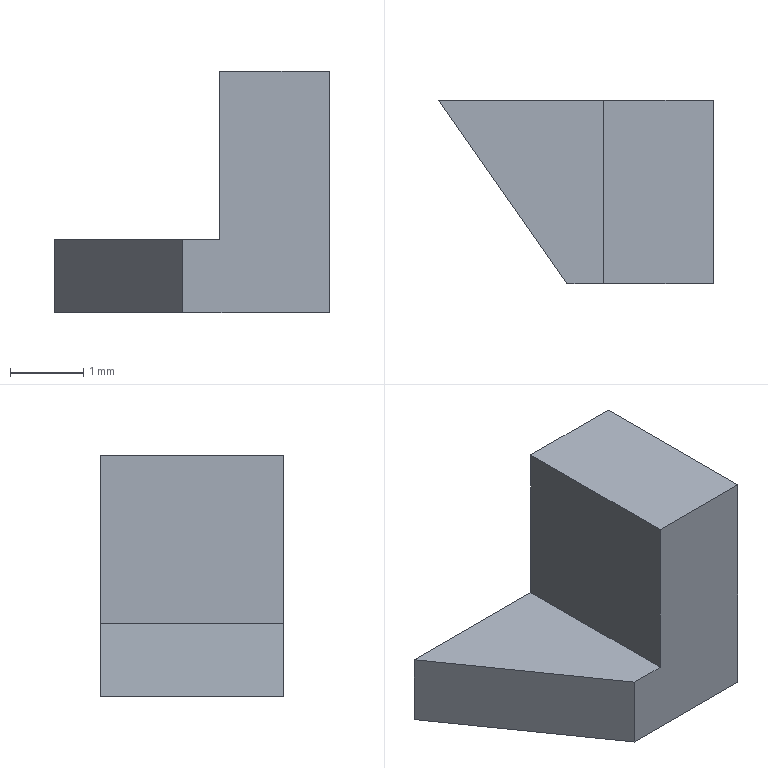Part | SolidWorks | features Extrusion 1, ICE 1 | 1 solid | 8 faces | box 3.751 x 2.5 x 3.3 mm | volume 15.813 mm3 | plane 8
STEP:
#1=CARTESIAN_POINT('',(0.,0.,0.));
#2=VERTEX_POINT('',#1);
#3=CARTESIAN_POINT('',(2.,0.,0.));
#4=VERTEX_POINT('',#3);
#5=CARTESIAN_POINT('',(2.,0.,0.));
#6=DIRECTION('',(1.,0.,0.));
#7=VECTOR('',#6,1000.);
#8=LINE('',#5,#7);
#9=EDGE_CURVE('',#2,#4,#8,.T.);
#10=ORIENTED_EDGE('',*,*,#9,.T.);
#11=CARTESIAN_POINT('',(2.,0.,3.3));
#12=VERTEX_POINT('',#11);
#13=CARTESIAN_POINT('',(2.,0.,1.));
#14=DIRECTION('',(0.,0.,-1.));
#15=VECTOR('',#14,1000.);
#16=LINE('',#13,#15);
#17=EDGE_CURVE('',#12,#4,#16,.T.);
#18=ORIENTED_EDGE('',*,*,#17,.F.);
#19=CARTESIAN_POINT('',(0.5,0.,3.3));
#20=VERTEX_POINT('',#19);
#21=CARTESIAN_POINT('',(2.,0.,3.3));
#22=DIRECTION('',(1.,0.,0.));
#23=VECTOR('',#22,1000.);
#24=LINE('',#21,#23);
#25=EDGE_CURVE('',#20,#12,#24,.T.);
#26=ORIENTED_EDGE('',*,*,#25,.F.);
#27=CARTESIAN_POINT('',(0.5,0.,1.));
#28=VERTEX_POINT('',#27);
#29=CARTESIAN_POINT('',(0.5,0.,3.3));
#30=DIRECTION('',(0.,0.,-1.));
#31=VECTOR('',#30,1000.);
#32=LINE('',#29,#31);
#33=EDGE_CURVE('',#20,#28,#32,.T.);
#34=ORIENTED_EDGE('',*,*,#33,.T.);
#35=CARTESIAN_POINT('',(0.,0.,1.));
#36=VERTEX_POINT('',#35);
#37=CARTESIAN_POINT('',(2.,0.,1.));
#38=DIRECTION('',(1.,0.,0.));
#39=VECTOR('',#38,1000.);
#40=LINE('',#37,#39);
#41=EDGE_CURVE('',#36,#28,#40,.T.);
#42=ORIENTED_EDGE('',*,*,#41,.F.);
#43=CARTESIAN_POINT('',(0.,0.,1.));
#44=DIRECTION('',(0.,0.,-1.));
#45=VECTOR('',#44,1000.);
#46=LINE('',#43,#45);
#47=EDGE_CURVE('',#36,#2,#46,.T.);
#48=ORIENTED_EDGE('',*,*,#47,.T.);
#49=EDGE_LOOP('',(#10,#18,#26,#34,#42,#48));
#50=FACE_OUTER_BOUND('',#49,.T.);
#51=CARTESIAN_POINT('',(2.,0.,1.));
#52=DIRECTION('',(0.,1.,0.));
#53=DIRECTION('',(-1.,0.,0.));
#54=AXIS2_PLACEMENT_3D('',#51,#52,#53);
#55=PLANE('',#54);
#56=ADVANCED_FACE('',(#50),#55,.F.);
#57=CARTESIAN_POINT('',(2.,2.5,0.));
#58=VERTEX_POINT('',#57);
#59=CARTESIAN_POINT('',(2.,2.5,0.));
#60=DIRECTION('',(0.,1.,0.));
#61=VECTOR('',#60,1000.);
#62=LINE('',#59,#61);
#63=EDGE_CURVE('',#4,#58,#62,.T.);
#64=ORIENTED_EDGE('',*,*,#63,.T.);
#65=CARTESIAN_POINT('',(2.,2.5,3.3));
#66=VERTEX_POINT('',#65);
#67=CARTESIAN_POINT('',(2.,2.5,1.));
#68=DIRECTION('',(0.,0.,-1.));
#69=VECTOR('',#68,1000.);
#70=LINE('',#67,#69);
#71=EDGE_CURVE('',#66,#58,#70,.T.);
#72=ORIENTED_EDGE('',*,*,#71,.F.);
#73=CARTESIAN_POINT('',(2.,2.5,3.3));
#74=DIRECTION('',(0.,1.,0.));
#75=VECTOR('',#74,1000.);
#76=LINE('',#73,#75);
#77=EDGE_CURVE('',#12,#66,#76,.T.);
#78=ORIENTED_EDGE('',*,*,#77,.F.);
#79=ORIENTED_EDGE('',*,*,#17,.T.);
#80=EDGE_LOOP('',(#64,#72,#78,#79));
#81=FACE_OUTER_BOUND('',#80,.T.);
#82=CARTESIAN_POINT('',(2.,2.5,1.));
#83=DIRECTION('',(-1.,0.,0.));
#84=DIRECTION('',(0.,0.,1.));
#85=AXIS2_PLACEMENT_3D('',#82,#83,#84);
#86=PLANE('',#85);
#87=ADVANCED_FACE('',(#81),#86,.F.);
#88=CARTESIAN_POINT('',(-1.751,2.5,0.));
#89=VERTEX_POINT('',#88);
#90=CARTESIAN_POINT('',(-1.751,2.5,0.));
#91=DIRECTION('',(-1.,0.,0.));
#92=VECTOR('',#91,1000.);
#93=LINE('',#90,#92);
#94=EDGE_CURVE('',#58,#89,#93,.T.);
#95=ORIENTED_EDGE('',*,*,#94,.T.);
#96=CARTESIAN_POINT('',(-1.751,2.5,1.));
#97=VERTEX_POINT('',#96);
#98=CARTESIAN_POINT('',(-1.751,2.5,1.));
#99=DIRECTION('',(0.,0.,-1.));
#100=VECTOR('',#99,1000.);
#101=LINE('',#98,#100);
#102=EDGE_CURVE('',#97,#89,#101,.T.);
#103=ORIENTED_EDGE('',*,*,#102,.F.);
#104=CARTESIAN_POINT('',(0.5,2.5,1.));
#105=VERTEX_POINT('',#104);
#106=CARTESIAN_POINT('',(-1.751,2.5,1.));
#107=DIRECTION('',(-1.,0.,0.));
#108=VECTOR('',#107,1000.);
#109=LINE('',#106,#108);
#110=EDGE_CURVE('',#105,#97,#109,.T.);
#111=ORIENTED_EDGE('',*,*,#110,.F.);
#112=CARTESIAN_POINT('',(0.5,2.5,3.3));
#113=VERTEX_POINT('',#112);
#114=CARTESIAN_POINT('',(0.5,2.5,3.3));
#115=DIRECTION('',(0.,0.,-1.));
#116=VECTOR('',#115,1000.);
#117=LINE('',#114,#116);
#118=EDGE_CURVE('',#113,#105,#117,.T.);
#119=ORIENTED_EDGE('',*,*,#118,.F.);
#120=CARTESIAN_POINT('',(2.,2.5,3.3));
#121=DIRECTION('',(-1.,0.,0.));
#122=VECTOR('',#121,1000.);
#123=LINE('',#120,#122);
#124=EDGE_CURVE('',#66,#113,#123,.T.);
#125=ORIENTED_EDGE('',*,*,#124,.F.);
#126=ORIENTED_EDGE('',*,*,#71,.T.);
#127=EDGE_LOOP('',(#95,#103,#111,#119,#125,#126));
#128=FACE_OUTER_BOUND('',#127,.T.);
#129=CARTESIAN_POINT('',(-1.751,2.5,1.));
#130=DIRECTION('',(0.,-1.,0.));
#131=DIRECTION('',(0.,0.,-1.));
#132=AXIS2_PLACEMENT_3D('',#129,#130,#131);
#133=PLANE('',#132);
#134=ADVANCED_FACE('',(#128),#133,.F.);
#135=CARTESIAN_POINT('',(0.,0.,0.));
#136=DIRECTION('',(0.5736,-0.8192,0.));
#137=VECTOR('',#136,1000.);
#138=LINE('',#135,#137);
#139=EDGE_CURVE('',#89,#2,#138,.T.);
#140=ORIENTED_EDGE('',*,*,#139,.T.);
#141=ORIENTED_EDGE('',*,*,#47,.F.);
#142=CARTESIAN_POINT('',(0.,0.,1.));
#143=DIRECTION('',(0.5736,-0.8192,0.));
#144=VECTOR('',#143,1000.);
#145=LINE('',#142,#144);
#146=EDGE_CURVE('',#97,#36,#145,.T.);
#147=ORIENTED_EDGE('',*,*,#146,.F.);
#148=ORIENTED_EDGE('',*,*,#102,.T.);
#149=EDGE_LOOP('',(#140,#141,#147,#148));
#150=FACE_OUTER_BOUND('',#149,.T.);
#151=CARTESIAN_POINT('',(0.,0.,1.));
#152=DIRECTION('',(0.8192,0.5736,0.));
#153=DIRECTION('',(-0.5736,0.8192,0.));
#154=AXIS2_PLACEMENT_3D('',#151,#152,#153);
#155=PLANE('',#154);
#156=ADVANCED_FACE('',(#150),#155,.F.);
#157=CARTESIAN_POINT('',(0.5,2.5,1.));
#158=DIRECTION('',(0.,-1.,0.));
#159=VECTOR('',#158,1000.);
#160=LINE('',#157,#159);
#161=EDGE_CURVE('',#105,#28,#160,.T.);
#162=ORIENTED_EDGE('',*,*,#161,.F.);
#163=ORIENTED_EDGE('',*,*,#110,.T.);
#164=ORIENTED_EDGE('',*,*,#146,.T.);
#165=ORIENTED_EDGE('',*,*,#41,.T.);
#166=EDGE_LOOP('',(#162,#163,#164,#165));
#167=FACE_OUTER_BOUND('',#166,.T.);
#168=CARTESIAN_POINT('',(0.,0.,1.));
#169=DIRECTION('',(0.,0.,1.));
#170=DIRECTION('',(1.,0.,0.));
#171=AXIS2_PLACEMENT_3D('',#168,#169,#170);
#172=PLANE('',#171);
#173=ADVANCED_FACE('',(#167),#172,.T.);
#174=ORIENTED_EDGE('',*,*,#9,.F.);
#175=ORIENTED_EDGE('',*,*,#139,.F.);
#176=ORIENTED_EDGE('',*,*,#94,.F.);
#177=ORIENTED_EDGE('',*,*,#63,.F.);
#178=EDGE_LOOP('',(#174,#175,#176,#177));
#179=FACE_OUTER_BOUND('',#178,.T.);
#180=CARTESIAN_POINT('',(0.,0.,0.));
#181=DIRECTION('',(0.,0.,1.));
#182=DIRECTION('',(1.,0.,0.));
#183=AXIS2_PLACEMENT_3D('',#180,#181,#182);
#184=PLANE('',#183);
#185=ADVANCED_FACE('',(#179),#184,.F.);
#186=ORIENTED_EDGE('',*,*,#161,.T.);
#187=ORIENTED_EDGE('',*,*,#33,.F.);
#188=CARTESIAN_POINT('',(0.5,2.5,3.3));
#189=DIRECTION('',(0.,-1.,0.));
#190=VECTOR('',#189,1000.);
#191=LINE('',#188,#190);
#192=EDGE_CURVE('',#113,#20,#191,.T.);
#193=ORIENTED_EDGE('',*,*,#192,.F.);
#194=ORIENTED_EDGE('',*,*,#118,.T.);
#195=EDGE_LOOP('',(#186,#187,#193,#194));
#196=FACE_OUTER_BOUND('',#195,.T.);
#197=CARTESIAN_POINT('',(0.5,2.5,3.3));
#198=DIRECTION('',(1.,0.,0.));
#199=DIRECTION('',(0.,1.,0.));
#200=AXIS2_PLACEMENT_3D('',#197,#198,#199);
#201=PLANE('',#200);
#202=ADVANCED_FACE('',(#196),#201,.F.);
#203=ORIENTED_EDGE('',*,*,#77,.T.);
#204=ORIENTED_EDGE('',*,*,#124,.T.);
#205=ORIENTED_EDGE('',*,*,#192,.T.);
#206=ORIENTED_EDGE('',*,*,#25,.T.);
#207=EDGE_LOOP('',(#203,#204,#205,#206));
#208=FACE_OUTER_BOUND('',#207,.T.);
#209=CARTESIAN_POINT('',(0.,0.,3.3));
#210=DIRECTION('',(0.,0.,-1.));
#211=DIRECTION('',(-1.,0.,0.));
#212=AXIS2_PLACEMENT_3D('',#209,#210,#211);
#213=PLANE('',#212);
#214=ADVANCED_FACE('',(#208),#213,.F.);
#215=CLOSED_SHELL('',(#56,#87,#134,#156,#173,#185,#202,#214));
#216=MANIFOLD_SOLID_BREP('',#215);
#217=CARTESIAN_POINT('',(0.,0.,0.));
#218=DIRECTION('',(0.,0.,1.));
#219=DIRECTION('',(1.,0.,0.));
#220=AXIS2_PLACEMENT_3D('',#217,#218,#219);
#221=(LENGTH_UNIT()NAMED_UNIT(*)SI_UNIT(.MILLI.,.METRE.));
#222=UNCERTAINTY_MEASURE_WITH_UNIT(LENGTH_MEASURE(0.00001),#221,'','');
#223=(NAMED_UNIT(*)PLANE_ANGLE_UNIT()SI_UNIT($,.RADIAN.));
#224=(NAMED_UNIT(*)SI_UNIT($,.STERADIAN.)SOLID_ANGLE_UNIT());
#225=(GEOMETRIC_REPRESENTATION_CONTEXT(3)GLOBAL_UNCERTAINTY_ASSIGNED_CONTEXT((#222))GLOBAL_UNIT_ASSIGNED_CONTEXT((#221,#223,#224))REPRESENTATION_CONTEXT('',''));
#226=ADVANCED_BREP_SHAPE_REPRESENTATION('',(#216,#220),#225);